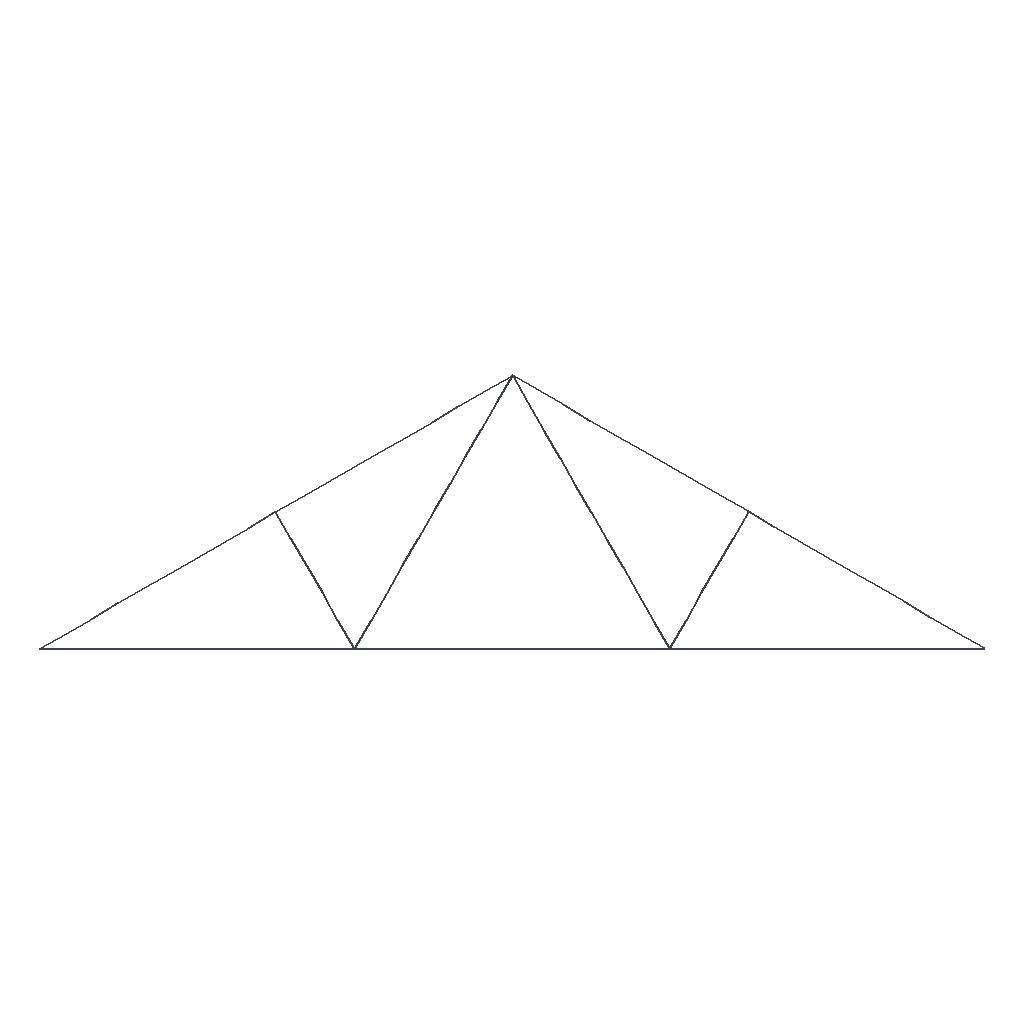Simulation study | abaqus
Set-up summary:
category,name,step,type,value,unit,region
solver,abaqus,,Abaqus/CAE 2024
units,mm-N-s-tonne (MPa),,inferred,E=200000 density=
analysis,Step-1,,static,time_period=1
mesh,nodes,,,92
mesh,elements,,,96
element_type,T3D2,,,96
material,Material-1,,E,200000
material,Material-1,,nu,0.3
section,Material-1,,solid section,,,_PickedSet2
load,Load-1,Step-1,concentrated force,"300000 [dir=(0, -1, 0)]",,_PickedSet7
bc,BC-1,Step-1,fixed,"[dofs=rx,ry,x,y,z n=5]",,_PickedSet4
bc,BC-2,Step-1,fixed,"[dofs=rx,ry,y,z n=4]",,_PickedSet5
Abaqus input file, long lists of numbers shortened:
*Heading
** Job name: deck Model name: Model-1
** Generated by: Abaqus/CAE 2024
*Preprint, echo=NO, model=NO, history=NO, contact=NO
**
** PARTS
**
*Part, name=Part-1
*Node
      1,   53293.598,   16455.846,           0.
      2,   54793.598,   19053.922,           0.
** (90 more lines like these left out)
*Element, type=T3D2
1,  2,  8
2,  8,  9
** (94 more lines like these left out)
*Nset, nset=_PickedSet2, internal, generate
  1,  92,   1
*Elset, elset=_PickedSet2, internal, generate
  1,  96,   1
** Section: Section-1
*Solid Section, elset=_PickedSet2, material=Material-1
100000.,
*End Part
**
**
** ASSEMBLY
**
*Assembly, name=Assembly
**
*Instance, name=Part-1-1, part=Part-1
-41293.598, -16455.845,           0.
*End Instance
**
*Nset, nset=_PickedSet4, internal, instance=Part-1-1
 7,
*Nset, nset=_PickedSet5, internal, instance=Part-1-1
 3,
*Nset, nset=_PickedSet7, internal, instance=Part-1-1
 1, 5
*End Assembly
**
** MATERIALS
**
*Material, name=Material-1
*Elastic
200000., 0.3
** ----------------------------------------------------------------
**
** STEP: Step-1
**
*Step, name=Step-1, nlgeom=NO
*Static, stabilize=0.0002, allsdtol=0.05, continue=NO
0.1, 1., 1e-05, 0.1
**
** BOUNDARY CONDITIONS
**
** Name: BC-1 Type: Displacement/Rotation
*Boundary
_PickedSet4, 1, 1
_PickedSet4, 2, 2
_PickedSet4, 3, 3
_PickedSet4, 4, 4
_PickedSet4, 5, 5
** Name: BC-2 Type: Displacement/Rotation
*Boundary
_PickedSet5, 2, 2
_PickedSet5, 3, 3
_PickedSet5, 4, 4
_PickedSet5, 5, 5
**
** LOADS
**
** Name: Load-1   Type: Concentrated force
*Cload
_PickedSet7, 2, -300000.
**
** OUTPUT REQUESTS
**
*Restart, write, frequency=0
**
** FIELD OUTPUT: F-Output-1
**
*Output, field, variable=PRESELECT
**
** HISTORY OUTPUT: H-Output-1
**
*Output, history, variable=PRESELECT
*End Step
Results summary:
result,odb.job_status,,,JOB_STATUS_COMPLETED_SUCCESSFULLY,"consistent, unstated (Abaqus has no unit system)"
result,steps[0].procedure,Step-1,,*STATIC,"consistent, unstated (Abaqus has no unit system)"
result,steps[0].time_period,Step-1,,1,"consistent, unstated (Abaqus has no unit system)"
result,steps[0].n_frames,Step-1,,11,"consistent, unstated (Abaqus has no unit system)"
result,steps[0].last_frame.id,Step-1,,10,"consistent, unstated (Abaqus has no unit system)"
result,steps[0].last_frame.value,Step-1,,1,"consistent, unstated (Abaqus has no unit system)"
result,steps[0].last_frame.description,Step-1,,Increment     10: Step Time =    1.000,"consistent, unstated (Abaqus has no unit system)"
result,steps[0].completed,Step-1,,True,"consistent, unstated (Abaqus has no unit system)"
result,steps[0].max_U_magnitude,Step-1,,1.104,"consistent, unstated (Abaqus has no unit system)"
result,steps[0].max_S_mises,Step-1,,5.997,"consistent, unstated (Abaqus has no unit system)"
result,steps[0].RF_sum[1],Step-1,,346.396,"consistent, unstated (Abaqus has no unit system)"
result,steps[0].RF_sum[2],Step-1,,599502,"consistent, unstated (Abaqus has no unit system)"
result,steps[0].RF_sum[3],Step-1,,0,"consistent, unstated (Abaqus has no unit system)"